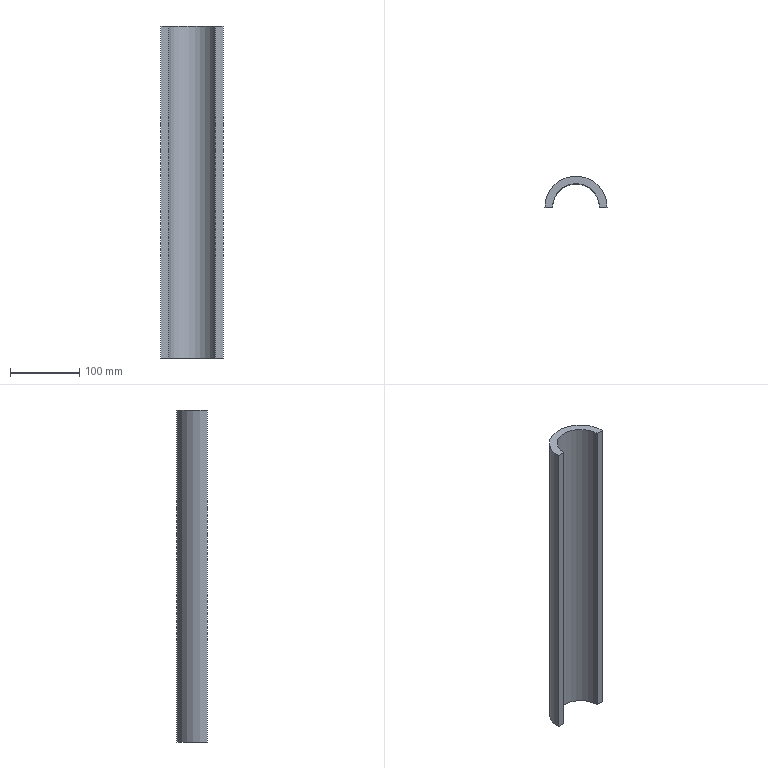Part | SolidWorks | features BaseBody 1 | 1 solid | 6 faces | box 90 x 45 x 481 mm | volume 656576 mm3 | plane 4 | cylinder 2 | commonest cylinder face diameters 68 x1 90 x1
STEP:
#1=CARTESIAN_POINT('',(-45.,-2.,-410.));
#2=VERTEX_POINT('',#1);
#3=CARTESIAN_POINT('',(-45.,-2.,71.));
#4=VERTEX_POINT('',#3);
#5=CARTESIAN_POINT('',(-45.,-2.,-410.));
#6=DIRECTION('',(0.,0.,1.));
#7=VECTOR('',#6,1000.);
#8=LINE('',#5,#7);
#9=EDGE_CURVE('',#2,#4,#8,.T.);
#10=ORIENTED_EDGE('',*,*,#9,.T.);
#11=CARTESIAN_POINT('',(45.,-2.,71.));
#12=VERTEX_POINT('',#11);
#13=CARTESIAN_POINT('',(0.,-2.,71.));
#14=DIRECTION('',(0.,0.,-1.));
#15=DIRECTION('',(1.,0.,0.));
#16=AXIS2_PLACEMENT_3D('',#13,#14,#15);
#17=CIRCLE('',#16,45.);
#18=EDGE_CURVE('',#4,#12,#17,.T.);
#19=ORIENTED_EDGE('',*,*,#18,.T.);
#20=CARTESIAN_POINT('',(45.,-2.,-410.));
#21=VERTEX_POINT('',#20);
#22=CARTESIAN_POINT('',(45.,-2.,-410.));
#23=DIRECTION('',(0.,0.,-1.));
#24=VECTOR('',#23,1000.);
#25=LINE('',#22,#24);
#26=EDGE_CURVE('',#12,#21,#25,.T.);
#27=ORIENTED_EDGE('',*,*,#26,.T.);
#28=CARTESIAN_POINT('',(0.,-2.,-410.));
#29=DIRECTION('',(0.,0.,1.));
#30=DIRECTION('',(1.,0.,0.));
#31=AXIS2_PLACEMENT_3D('',#28,#29,#30);
#32=CIRCLE('',#31,45.);
#33=EDGE_CURVE('',#21,#2,#32,.T.);
#34=ORIENTED_EDGE('',*,*,#33,.T.);
#35=EDGE_LOOP('',(#10,#19,#27,#34));
#36=FACE_OUTER_BOUND('',#35,.T.);
#37=CARTESIAN_POINT('',(0.,-2.,-410.));
#38=DIRECTION('',(0.,0.,1.));
#39=DIRECTION('',(1.,0.,0.));
#40=AXIS2_PLACEMENT_3D('',#37,#38,#39);
#41=CYLINDRICAL_SURFACE('',#40,45.);
#42=ADVANCED_FACE('',(#36),#41,.T.);
#43=CARTESIAN_POINT('',(-34.,-2.,71.));
#44=VERTEX_POINT('',#43);
#45=CARTESIAN_POINT('',(0.,-2.,71.));
#46=DIRECTION('',(1.,0.,0.));
#47=VECTOR('',#46,1000.);
#48=LINE('',#45,#47);
#49=EDGE_CURVE('',#4,#44,#48,.T.);
#50=ORIENTED_EDGE('',*,*,#49,.T.);
#51=CARTESIAN_POINT('',(34.,-2.,71.));
#52=VERTEX_POINT('',#51);
#53=CARTESIAN_POINT('',(0.,-2.,71.));
#54=DIRECTION('',(0.,0.,-1.));
#55=DIRECTION('',(1.,0.,0.));
#56=AXIS2_PLACEMENT_3D('',#53,#54,#55);
#57=CIRCLE('',#56,34.);
#58=EDGE_CURVE('',#44,#52,#57,.T.);
#59=ORIENTED_EDGE('',*,*,#58,.T.);
#60=CARTESIAN_POINT('',(0.,-2.,71.));
#61=DIRECTION('',(1.,0.,0.));
#62=VECTOR('',#61,1000.);
#63=LINE('',#60,#62);
#64=EDGE_CURVE('',#52,#12,#63,.T.);
#65=ORIENTED_EDGE('',*,*,#64,.T.);
#66=ORIENTED_EDGE('',*,*,#18,.F.);
#67=EDGE_LOOP('',(#50,#59,#65,#66));
#68=FACE_OUTER_BOUND('',#67,.T.);
#69=CARTESIAN_POINT('',(0.,20.528,71.));
#70=DIRECTION('',(0.,0.,1.));
#71=DIRECTION('',(1.,0.,0.));
#72=AXIS2_PLACEMENT_3D('',#69,#70,#71);
#73=PLANE('',#72);
#74=ADVANCED_FACE('',(#68),#73,.T.);
#75=CARTESIAN_POINT('',(-34.,-2.,-410.));
#76=VERTEX_POINT('',#75);
#77=CARTESIAN_POINT('',(-34.,-2.,-169.5));
#78=DIRECTION('',(0.,0.,-1.));
#79=VECTOR('',#78,1000.);
#80=LINE('',#77,#79);
#81=EDGE_CURVE('',#44,#76,#80,.T.);
#82=ORIENTED_EDGE('',*,*,#81,.F.);
#83=ORIENTED_EDGE('',*,*,#49,.F.);
#84=ORIENTED_EDGE('',*,*,#9,.F.);
#85=CARTESIAN_POINT('',(-39.5,-2.,-410.));
#86=DIRECTION('',(-1.,0.,0.));
#87=VECTOR('',#86,1000.);
#88=LINE('',#85,#87);
#89=EDGE_CURVE('',#76,#2,#88,.T.);
#90=ORIENTED_EDGE('',*,*,#89,.F.);
#91=EDGE_LOOP('',(#82,#83,#84,#90));
#92=FACE_OUTER_BOUND('',#91,.T.);
#93=CARTESIAN_POINT('',(-39.5,-2.,-169.5));
#94=DIRECTION('',(0.,1.,0.));
#95=DIRECTION('',(0.,0.,1.));
#96=AXIS2_PLACEMENT_3D('',#93,#94,#95);
#97=PLANE('',#96);
#98=ADVANCED_FACE('',(#92),#97,.F.);
#99=ORIENTED_EDGE('',*,*,#89,.T.);
#100=ORIENTED_EDGE('',*,*,#33,.F.);
#101=CARTESIAN_POINT('',(34.,-2.,-410.));
#102=VERTEX_POINT('',#101);
#103=CARTESIAN_POINT('',(0.,-2.,-410.));
#104=DIRECTION('',(1.,0.,0.));
#105=VECTOR('',#104,1000.);
#106=LINE('',#103,#105);
#107=EDGE_CURVE('',#102,#21,#106,.T.);
#108=ORIENTED_EDGE('',*,*,#107,.F.);
#109=CARTESIAN_POINT('',(0.,-2.,-410.));
#110=DIRECTION('',(0.,0.,-1.));
#111=DIRECTION('',(1.,0.,0.));
#112=AXIS2_PLACEMENT_3D('',#109,#110,#111);
#113=CIRCLE('',#112,34.);
#114=EDGE_CURVE('',#76,#102,#113,.T.);
#115=ORIENTED_EDGE('',*,*,#114,.F.);
#116=EDGE_LOOP('',(#99,#100,#108,#115));
#117=FACE_OUTER_BOUND('',#116,.T.);
#118=CARTESIAN_POINT('',(0.,20.528,-410.));
#119=DIRECTION('',(0.,0.,1.));
#120=DIRECTION('',(1.,0.,0.));
#121=AXIS2_PLACEMENT_3D('',#118,#119,#120);
#122=PLANE('',#121);
#123=ADVANCED_FACE('',(#117),#122,.F.);
#124=ORIENTED_EDGE('',*,*,#26,.F.);
#125=ORIENTED_EDGE('',*,*,#64,.F.);
#126=CARTESIAN_POINT('',(34.,-2.,-169.5));
#127=DIRECTION('',(0.,0.,1.));
#128=VECTOR('',#127,1000.);
#129=LINE('',#126,#128);
#130=EDGE_CURVE('',#102,#52,#129,.T.);
#131=ORIENTED_EDGE('',*,*,#130,.F.);
#132=ORIENTED_EDGE('',*,*,#107,.T.);
#133=EDGE_LOOP('',(#124,#125,#131,#132));
#134=FACE_OUTER_BOUND('',#133,.T.);
#135=CARTESIAN_POINT('',(39.5,-2.,-169.5));
#136=DIRECTION('',(0.,1.,0.));
#137=DIRECTION('',(0.,0.,1.));
#138=AXIS2_PLACEMENT_3D('',#135,#136,#137);
#139=PLANE('',#138);
#140=ADVANCED_FACE('',(#134),#139,.F.);
#141=ORIENTED_EDGE('',*,*,#81,.T.);
#142=ORIENTED_EDGE('',*,*,#114,.T.);
#143=ORIENTED_EDGE('',*,*,#130,.T.);
#144=ORIENTED_EDGE('',*,*,#58,.F.);
#145=EDGE_LOOP('',(#141,#142,#143,#144));
#146=FACE_OUTER_BOUND('',#145,.T.);
#147=CARTESIAN_POINT('',(0.,-2.,-410.));
#148=DIRECTION('',(0.,0.,1.));
#149=DIRECTION('',(1.,0.,0.));
#150=AXIS2_PLACEMENT_3D('',#147,#148,#149);
#151=CYLINDRICAL_SURFACE('',#150,34.);
#152=ADVANCED_FACE('',(#146),#151,.F.);
#153=CLOSED_SHELL('',(#42,#74,#98,#123,#140,#152));
#154=MANIFOLD_SOLID_BREP('',#153);
#155=CARTESIAN_POINT('',(0.,0.,0.));
#156=DIRECTION('',(0.,0.,1.));
#157=DIRECTION('',(1.,0.,0.));
#158=AXIS2_PLACEMENT_3D('',#155,#156,#157);
#159=(LENGTH_UNIT()NAMED_UNIT(*)SI_UNIT(.MILLI.,.METRE.));
#160=UNCERTAINTY_MEASURE_WITH_UNIT(LENGTH_MEASURE(0.00001),#159,'','');
#161=(NAMED_UNIT(*)PLANE_ANGLE_UNIT()SI_UNIT($,.RADIAN.));
#162=(NAMED_UNIT(*)SI_UNIT($,.STERADIAN.)SOLID_ANGLE_UNIT());
#163=(GEOMETRIC_REPRESENTATION_CONTEXT(3)GLOBAL_UNCERTAINTY_ASSIGNED_CONTEXT((#160))GLOBAL_UNIT_ASSIGNED_CONTEXT((#159,#161,#162))REPRESENTATION_CONTEXT('',''));
#164=ADVANCED_BREP_SHAPE_REPRESENTATION('',(#154,#158),#163);